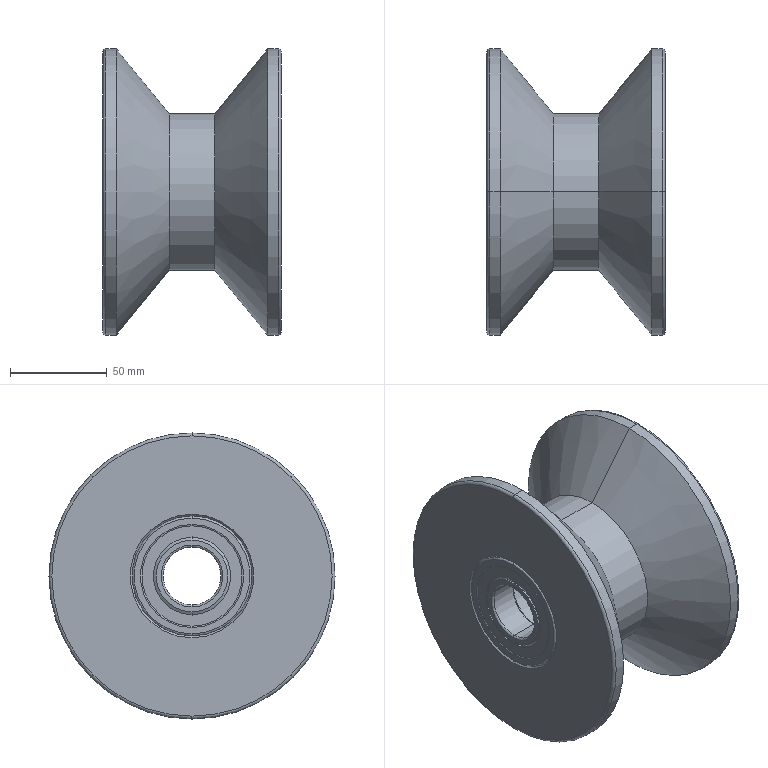Part | SolidWorks | features BaseBody 33 | 33 solids | 416 faces | box 92.206 x 148 x 148 mm | volume 771498 mm3 | cylinder 152 | sphere 120 | plane 76 | torus 48 | cone 20 | commonest cylinder face diameters 44.4 x54 47.6 x54 37.111 x8 40.667 x8 51.333 x8 62 x8